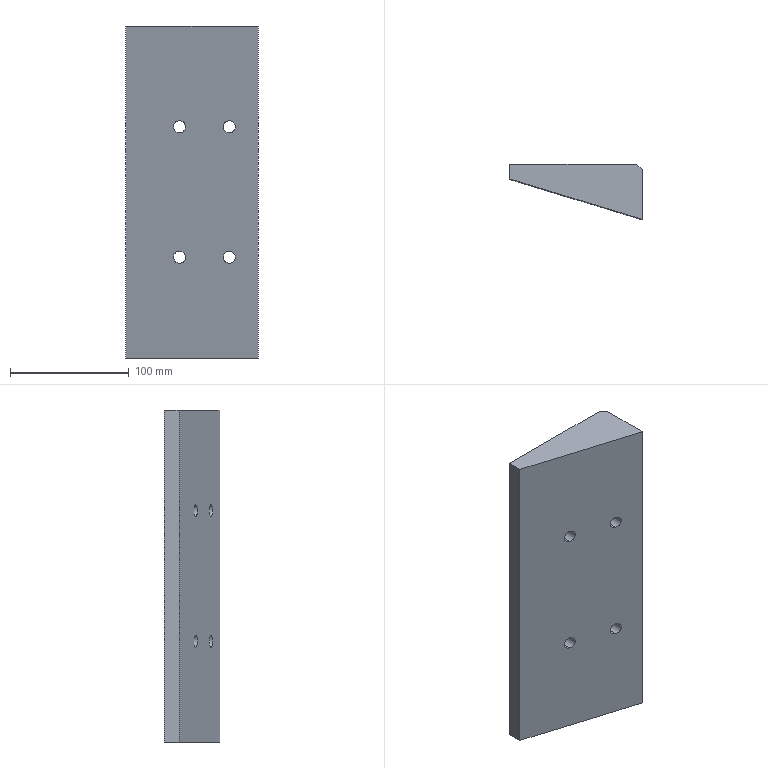Part | SolidWorks | features Extrusion 1, HoleWzd 1 | 1 solid | 15 faces | box 112 x 46.7 x 280 mm | volume 914034 mm3 | cylinder 8 | plane 7 | commonest cylinder face diameters 10.2 x8
STEP:
#1=CARTESIAN_POINT('',(45.5,-13.894,189.9));
#2=VERTEX_POINT('',#1);
#3=CARTESIAN_POINT('',(45.5,-13.894,200.1));
#4=VERTEX_POINT('',#3);
#5=CARTESIAN_POINT('',(45.5,-13.894,189.9));
#6=CARTESIAN_POINT('',(35.3,-10.779,189.9));
#7=CARTESIAN_POINT('',(35.3,-10.779,200.1));
#8=CARTESIAN_POINT('',(45.5,-13.894,200.1));
#9=(BOUNDED_CURVE()B_SPLINE_CURVE(3,(#5,#6,#7,#8),.UNSPECIFIED.,.F.,.T.)B_SPLINE_CURVE_WITH_KNOTS((4,4),(4.712,7.854),.UNSPECIFIED.)CURVE()GEOMETRIC_REPRESENTATION_ITEM()RATIONAL_B_SPLINE_CURVE((1.,0.3333,0.3333,1.))REPRESENTATION_ITEM(''));
#10=EDGE_CURVE('',#2,#4,#9,.T.);
#11=ORIENTED_EDGE('',*,*,#10,.F.);
#12=CARTESIAN_POINT('',(45.5,12.5,189.9));
#13=VERTEX_POINT('',#12);
#14=CARTESIAN_POINT('',(45.5,12.5,189.9));
#15=DIRECTION('',(0.,1.,0.));
#16=VECTOR('',#15,1000.);
#17=LINE('',#14,#16);
#18=EDGE_CURVE('',#2,#13,#17,.T.);
#19=ORIENTED_EDGE('',*,*,#18,.T.);
#20=CARTESIAN_POINT('',(45.5,12.5,200.1));
#21=VERTEX_POINT('',#20);
#22=CARTESIAN_POINT('',(45.5,12.5,195.));
#23=DIRECTION('',(0.,1.,0.));
#24=DIRECTION('',(0.,0.,1.));
#25=AXIS2_PLACEMENT_3D('',#22,#23,#24);
#26=CIRCLE('',#25,5.1);
#27=EDGE_CURVE('',#13,#21,#26,.T.);
#28=ORIENTED_EDGE('',*,*,#27,.T.);
#29=CARTESIAN_POINT('',(45.5,12.5,200.1));
#30=DIRECTION('',(0.,1.,0.));
#31=VECTOR('',#30,1000.);
#32=LINE('',#29,#31);
#33=EDGE_CURVE('',#4,#21,#32,.T.);
#34=ORIENTED_EDGE('',*,*,#33,.F.);
#35=EDGE_LOOP('',(#11,#19,#28,#34));
#36=FACE_OUTER_BOUND('',#35,.T.);
#37=CARTESIAN_POINT('',(45.5,12.5,195.));
#38=DIRECTION('',(0.,1.,0.));
#39=DIRECTION('',(0.,0.,1.));
#40=AXIS2_PLACEMENT_3D('',#37,#38,#39);
#41=CYLINDRICAL_SURFACE('',#40,5.1);
#42=ADVANCED_FACE('',(#36),#41,.F.);
#43=CARTESIAN_POINT('',(45.5,-13.894,79.9));
#44=VERTEX_POINT('',#43);
#45=CARTESIAN_POINT('',(45.5,-13.894,90.1));
#46=VERTEX_POINT('',#45);
#47=CARTESIAN_POINT('',(45.5,-13.894,79.9));
#48=CARTESIAN_POINT('',(35.3,-10.779,79.9));
#49=CARTESIAN_POINT('',(35.3,-10.779,90.1));
#50=CARTESIAN_POINT('',(45.5,-13.894,90.1));
#51=(BOUNDED_CURVE()B_SPLINE_CURVE(3,(#47,#48,#49,#50),.UNSPECIFIED.,.F.,.F.)B_SPLINE_CURVE_WITH_KNOTS((4,4),(4.712,7.854),.UNSPECIFIED.)CURVE()GEOMETRIC_REPRESENTATION_ITEM()RATIONAL_B_SPLINE_CURVE((1.,0.3333,0.3333,1.))REPRESENTATION_ITEM(''));
#52=EDGE_CURVE('',#44,#46,#51,.T.);
#53=ORIENTED_EDGE('',*,*,#52,.F.);
#54=CARTESIAN_POINT('',(45.5,12.5,79.9));
#55=VERTEX_POINT('',#54);
#56=CARTESIAN_POINT('',(45.5,12.5,79.9));
#57=DIRECTION('',(0.,1.,0.));
#58=VECTOR('',#57,1000.);
#59=LINE('',#56,#58);
#60=EDGE_CURVE('',#44,#55,#59,.T.);
#61=ORIENTED_EDGE('',*,*,#60,.T.);
#62=CARTESIAN_POINT('',(45.5,12.5,90.1));
#63=VERTEX_POINT('',#62);
#64=CARTESIAN_POINT('',(45.5,12.5,85.));
#65=DIRECTION('',(0.,1.,0.));
#66=DIRECTION('',(0.,0.,1.));
#67=AXIS2_PLACEMENT_3D('',#64,#65,#66);
#68=CIRCLE('',#67,5.1);
#69=EDGE_CURVE('',#55,#63,#68,.T.);
#70=ORIENTED_EDGE('',*,*,#69,.T.);
#71=CARTESIAN_POINT('',(45.5,12.5,90.1));
#72=DIRECTION('',(0.,1.,0.));
#73=VECTOR('',#72,1000.);
#74=LINE('',#71,#73);
#75=EDGE_CURVE('',#46,#63,#74,.T.);
#76=ORIENTED_EDGE('',*,*,#75,.F.);
#77=EDGE_LOOP('',(#53,#61,#70,#76));
#78=FACE_OUTER_BOUND('',#77,.T.);
#79=CARTESIAN_POINT('',(45.5,12.5,85.));
#80=DIRECTION('',(0.,1.,0.));
#81=DIRECTION('',(0.,0.,1.));
#82=AXIS2_PLACEMENT_3D('',#79,#80,#81);
#83=CYLINDRICAL_SURFACE('',#82,5.1);
#84=ADVANCED_FACE('',(#78),#83,.F.);
#85=CARTESIAN_POINT('',(87.5,-26.719,79.9));
#86=VERTEX_POINT('',#85);
#87=CARTESIAN_POINT('',(87.5,-26.719,90.1));
#88=VERTEX_POINT('',#87);
#89=CARTESIAN_POINT('',(87.5,-26.719,79.9));
#90=CARTESIAN_POINT('',(77.3,-23.604,79.9));
#91=CARTESIAN_POINT('',(77.3,-23.604,90.1));
#92=CARTESIAN_POINT('',(87.5,-26.719,90.1));
#93=(BOUNDED_CURVE()B_SPLINE_CURVE(3,(#89,#90,#91,#92),.UNSPECIFIED.,.F.,.F.)B_SPLINE_CURVE_WITH_KNOTS((4,4),(4.712,7.854),.UNSPECIFIED.)CURVE()GEOMETRIC_REPRESENTATION_ITEM()RATIONAL_B_SPLINE_CURVE((1.,0.3333,0.3333,1.))REPRESENTATION_ITEM(''));
#94=EDGE_CURVE('',#86,#88,#93,.T.);
#95=ORIENTED_EDGE('',*,*,#94,.F.);
#96=CARTESIAN_POINT('',(87.5,12.5,79.9));
#97=VERTEX_POINT('',#96);
#98=CARTESIAN_POINT('',(87.5,12.5,79.9));
#99=DIRECTION('',(0.,1.,0.));
#100=VECTOR('',#99,1000.);
#101=LINE('',#98,#100);
#102=EDGE_CURVE('',#86,#97,#101,.T.);
#103=ORIENTED_EDGE('',*,*,#102,.T.);
#104=CARTESIAN_POINT('',(87.5,12.5,90.1));
#105=VERTEX_POINT('',#104);
#106=CARTESIAN_POINT('',(87.5,12.5,85.));
#107=DIRECTION('',(0.,1.,0.));
#108=DIRECTION('',(0.,0.,1.));
#109=AXIS2_PLACEMENT_3D('',#106,#107,#108);
#110=CIRCLE('',#109,5.1);
#111=EDGE_CURVE('',#97,#105,#110,.T.);
#112=ORIENTED_EDGE('',*,*,#111,.T.);
#113=CARTESIAN_POINT('',(87.5,12.5,90.1));
#114=DIRECTION('',(0.,1.,0.));
#115=VECTOR('',#114,1000.);
#116=LINE('',#113,#115);
#117=EDGE_CURVE('',#88,#105,#116,.T.);
#118=ORIENTED_EDGE('',*,*,#117,.F.);
#119=EDGE_LOOP('',(#95,#103,#112,#118));
#120=FACE_OUTER_BOUND('',#119,.T.);
#121=CARTESIAN_POINT('',(87.5,12.5,85.));
#122=DIRECTION('',(0.,1.,0.));
#123=DIRECTION('',(0.,0.,1.));
#124=AXIS2_PLACEMENT_3D('',#121,#122,#123);
#125=CYLINDRICAL_SURFACE('',#124,5.1);
#126=ADVANCED_FACE('',(#120),#125,.F.);
#127=CARTESIAN_POINT('',(87.5,-26.719,189.9));
#128=VERTEX_POINT('',#127);
#129=CARTESIAN_POINT('',(87.5,-26.719,200.1));
#130=VERTEX_POINT('',#129);
#131=CARTESIAN_POINT('',(87.5,-26.719,189.9));
#132=CARTESIAN_POINT('',(77.3,-23.604,189.9));
#133=CARTESIAN_POINT('',(77.3,-23.604,200.1));
#134=CARTESIAN_POINT('',(87.5,-26.719,200.1));
#135=(BOUNDED_CURVE()B_SPLINE_CURVE(3,(#131,#132,#133,#134),.UNSPECIFIED.,.F.,.T.)B_SPLINE_CURVE_WITH_KNOTS((4,4),(4.712,7.854),.UNSPECIFIED.)CURVE()GEOMETRIC_REPRESENTATION_ITEM()RATIONAL_B_SPLINE_CURVE((1.,0.3333,0.3333,1.))REPRESENTATION_ITEM(''));
#136=EDGE_CURVE('',#128,#130,#135,.T.);
#137=ORIENTED_EDGE('',*,*,#136,.F.);
#138=CARTESIAN_POINT('',(87.5,12.5,189.9));
#139=VERTEX_POINT('',#138);
#140=CARTESIAN_POINT('',(87.5,12.5,189.9));
#141=DIRECTION('',(0.,1.,0.));
#142=VECTOR('',#141,1000.);
#143=LINE('',#140,#142);
#144=EDGE_CURVE('',#128,#139,#143,.T.);
#145=ORIENTED_EDGE('',*,*,#144,.T.);
#146=CARTESIAN_POINT('',(87.5,12.5,200.1));
#147=VERTEX_POINT('',#146);
#148=CARTESIAN_POINT('',(87.5,12.5,195.));
#149=DIRECTION('',(0.,1.,0.));
#150=DIRECTION('',(0.,0.,1.));
#151=AXIS2_PLACEMENT_3D('',#148,#149,#150);
#152=CIRCLE('',#151,5.1);
#153=EDGE_CURVE('',#139,#147,#152,.T.);
#154=ORIENTED_EDGE('',*,*,#153,.T.);
#155=CARTESIAN_POINT('',(87.5,12.5,200.1));
#156=DIRECTION('',(0.,1.,0.));
#157=VECTOR('',#156,1000.);
#158=LINE('',#155,#157);
#159=EDGE_CURVE('',#130,#147,#158,.T.);
#160=ORIENTED_EDGE('',*,*,#159,.F.);
#161=EDGE_LOOP('',(#137,#145,#154,#160));
#162=FACE_OUTER_BOUND('',#161,.T.);
#163=CARTESIAN_POINT('',(87.5,12.5,195.));
#164=DIRECTION('',(0.,1.,0.));
#165=DIRECTION('',(0.,0.,1.));
#166=AXIS2_PLACEMENT_3D('',#163,#164,#165);
#167=CYLINDRICAL_SURFACE('',#166,5.1);
#168=ADVANCED_FACE('',(#162),#167,.F.);
#169=CARTESIAN_POINT('',(45.5,-13.894,200.1));
#170=CARTESIAN_POINT('',(55.7,-17.008,200.1));
#171=CARTESIAN_POINT('',(55.7,-17.008,189.9));
#172=CARTESIAN_POINT('',(45.5,-13.894,189.9));
#173=(BOUNDED_CURVE()B_SPLINE_CURVE(3,(#169,#170,#171,#172),.UNSPECIFIED.,.F.,.T.)B_SPLINE_CURVE_WITH_KNOTS((4,4),(1.571,4.712),.UNSPECIFIED.)CURVE()GEOMETRIC_REPRESENTATION_ITEM()RATIONAL_B_SPLINE_CURVE((1.,0.3333,0.3333,1.))REPRESENTATION_ITEM(''));
#174=EDGE_CURVE('',#4,#2,#173,.T.);
#175=ORIENTED_EDGE('',*,*,#174,.T.);
#176=ORIENTED_EDGE('',*,*,#10,.T.);
#177=EDGE_LOOP('',(#175,#176));
#178=FACE_BOUND('',#177,.T.);
#179=CARTESIAN_POINT('',(45.5,-13.894,90.1));
#180=CARTESIAN_POINT('',(55.7,-17.008,90.1));
#181=CARTESIAN_POINT('',(55.7,-17.008,79.9));
#182=CARTESIAN_POINT('',(45.5,-13.894,79.9));
#183=(BOUNDED_CURVE()B_SPLINE_CURVE(3,(#179,#180,#181,#182),.UNSPECIFIED.,.F.,.F.)B_SPLINE_CURVE_WITH_KNOTS((4,4),(1.571,4.712),.UNSPECIFIED.)CURVE()GEOMETRIC_REPRESENTATION_ITEM()RATIONAL_B_SPLINE_CURVE((1.,0.3333,0.3333,1.))REPRESENTATION_ITEM(''));
#184=EDGE_CURVE('',#46,#44,#183,.T.);
#185=ORIENTED_EDGE('',*,*,#184,.T.);
#186=ORIENTED_EDGE('',*,*,#52,.T.);
#187=EDGE_LOOP('',(#185,#186));
#188=FACE_BOUND('',#187,.T.);
#189=CARTESIAN_POINT('',(87.5,-26.719,90.1));
#190=CARTESIAN_POINT('',(97.7,-29.833,90.1));
#191=CARTESIAN_POINT('',(97.7,-29.833,79.9));
#192=CARTESIAN_POINT('',(87.5,-26.719,79.9));
#193=(BOUNDED_CURVE()B_SPLINE_CURVE(3,(#189,#190,#191,#192),.UNSPECIFIED.,.F.,.T.)B_SPLINE_CURVE_WITH_KNOTS((4,4),(1.571,4.712),.UNSPECIFIED.)CURVE()GEOMETRIC_REPRESENTATION_ITEM()RATIONAL_B_SPLINE_CURVE((1.,0.3333,0.3333,1.))REPRESENTATION_ITEM(''));
#194=EDGE_CURVE('',#88,#86,#193,.T.);
#195=ORIENTED_EDGE('',*,*,#194,.T.);
#196=ORIENTED_EDGE('',*,*,#94,.T.);
#197=EDGE_LOOP('',(#195,#196));
#198=FACE_BOUND('',#197,.T.);
#199=CARTESIAN_POINT('',(87.5,-26.719,200.1));
#200=CARTESIAN_POINT('',(97.7,-29.833,200.1));
#201=CARTESIAN_POINT('',(97.7,-29.833,189.9));
#202=CARTESIAN_POINT('',(87.5,-26.719,189.9));
#203=(BOUNDED_CURVE()B_SPLINE_CURVE(3,(#199,#200,#201,#202),.UNSPECIFIED.,.F.,.T.)B_SPLINE_CURVE_WITH_KNOTS((4,4),(1.571,4.712),.UNSPECIFIED.)CURVE()GEOMETRIC_REPRESENTATION_ITEM()RATIONAL_B_SPLINE_CURVE((1.,0.3333,0.3333,1.))REPRESENTATION_ITEM(''));
#204=EDGE_CURVE('',#130,#128,#203,.T.);
#205=ORIENTED_EDGE('',*,*,#204,.T.);
#206=ORIENTED_EDGE('',*,*,#136,.T.);
#207=EDGE_LOOP('',(#205,#206));
#208=FACE_BOUND('',#207,.T.);
#209=CARTESIAN_POINT('',(0.,0.,0.));
#210=VERTEX_POINT('',#209);
#211=CARTESIAN_POINT('',(112.,-34.2,0.));
#212=VERTEX_POINT('',#211);
#213=CARTESIAN_POINT('',(112.,-34.2,0.));
#214=DIRECTION('',(0.9564,-0.292,0.));
#215=VECTOR('',#214,1000.);
#216=LINE('',#213,#215);
#217=EDGE_CURVE('',#210,#212,#216,.T.);
#218=ORIENTED_EDGE('',*,*,#217,.T.);
#219=CARTESIAN_POINT('',(112.,-34.2,280.));
#220=VERTEX_POINT('',#219);
#221=CARTESIAN_POINT('',(112.,-34.2,280.));
#222=DIRECTION('',(0.,0.,-1.));
#223=VECTOR('',#222,1000.);
#224=LINE('',#221,#223);
#225=EDGE_CURVE('',#220,#212,#224,.T.);
#226=ORIENTED_EDGE('',*,*,#225,.F.);
#227=CARTESIAN_POINT('',(0.,0.,280.));
#228=VERTEX_POINT('',#227);
#229=CARTESIAN_POINT('',(112.,-34.2,280.));
#230=DIRECTION('',(0.9564,-0.292,0.));
#231=VECTOR('',#230,1000.);
#232=LINE('',#229,#231);
#233=EDGE_CURVE('',#228,#220,#232,.T.);
#234=ORIENTED_EDGE('',*,*,#233,.F.);
#235=CARTESIAN_POINT('',(0.,0.,280.));
#236=DIRECTION('',(0.,0.,-1.));
#237=VECTOR('',#236,1000.);
#238=LINE('',#235,#237);
#239=EDGE_CURVE('',#228,#210,#238,.T.);
#240=ORIENTED_EDGE('',*,*,#239,.T.);
#241=EDGE_LOOP('',(#218,#226,#234,#240));
#242=FACE_OUTER_BOUND('',#241,.T.);
#243=CARTESIAN_POINT('',(112.,-34.2,280.));
#244=DIRECTION('',(0.292,0.9564,0.));
#245=DIRECTION('',(-0.9564,0.292,0.));
#246=AXIS2_PLACEMENT_3D('',#243,#244,#245);
#247=PLANE('',#246);
#248=ADVANCED_FACE('',(#178,#188,#198,#208,#242),#247,.F.);
#249=CARTESIAN_POINT('',(112.,7.5,0.));
#250=VERTEX_POINT('',#249);
#251=CARTESIAN_POINT('',(112.,7.5,0.));
#252=DIRECTION('',(0.,1.,0.));
#253=VECTOR('',#252,1000.);
#254=LINE('',#251,#253);
#255=EDGE_CURVE('',#212,#250,#254,.T.);
#256=ORIENTED_EDGE('',*,*,#255,.T.);
#257=CARTESIAN_POINT('',(112.,7.5,280.));
#258=VERTEX_POINT('',#257);
#259=CARTESIAN_POINT('',(112.,7.5,280.));
#260=DIRECTION('',(0.,0.,-1.));
#261=VECTOR('',#260,1000.);
#262=LINE('',#259,#261);
#263=EDGE_CURVE('',#258,#250,#262,.T.);
#264=ORIENTED_EDGE('',*,*,#263,.F.);
#265=CARTESIAN_POINT('',(112.,7.5,280.));
#266=DIRECTION('',(0.,1.,0.));
#267=VECTOR('',#266,1000.);
#268=LINE('',#265,#267);
#269=EDGE_CURVE('',#220,#258,#268,.T.);
#270=ORIENTED_EDGE('',*,*,#269,.F.);
#271=ORIENTED_EDGE('',*,*,#225,.T.);
#272=EDGE_LOOP('',(#256,#264,#270,#271));
#273=FACE_OUTER_BOUND('',#272,.T.);
#274=CARTESIAN_POINT('',(112.,7.5,280.));
#275=DIRECTION('',(-1.,0.,0.));
#276=DIRECTION('',(0.,0.,1.));
#277=AXIS2_PLACEMENT_3D('',#274,#275,#276);
#278=PLANE('',#277);
#279=ADVANCED_FACE('',(#273),#278,.F.);
#280=CARTESIAN_POINT('',(107.,12.5,0.));
#281=VERTEX_POINT('',#280);
#282=CARTESIAN_POINT('',(107.,12.5,0.));
#283=DIRECTION('',(-0.7071,0.7071,0.));
#284=VECTOR('',#283,1000.);
#285=LINE('',#282,#284);
#286=EDGE_CURVE('',#250,#281,#285,.T.);
#287=ORIENTED_EDGE('',*,*,#286,.T.);
#288=CARTESIAN_POINT('',(107.,12.5,280.));
#289=VERTEX_POINT('',#288);
#290=CARTESIAN_POINT('',(107.,12.5,280.));
#291=DIRECTION('',(0.,0.,-1.));
#292=VECTOR('',#291,1000.);
#293=LINE('',#290,#292);
#294=EDGE_CURVE('',#289,#281,#293,.T.);
#295=ORIENTED_EDGE('',*,*,#294,.F.);
#296=CARTESIAN_POINT('',(107.,12.5,280.));
#297=DIRECTION('',(-0.7071,0.7071,0.));
#298=VECTOR('',#297,1000.);
#299=LINE('',#296,#298);
#300=EDGE_CURVE('',#258,#289,#299,.T.);
#301=ORIENTED_EDGE('',*,*,#300,.F.);
#302=ORIENTED_EDGE('',*,*,#263,.T.);
#303=EDGE_LOOP('',(#287,#295,#301,#302));
#304=FACE_OUTER_BOUND('',#303,.T.);
#305=CARTESIAN_POINT('',(107.,12.5,280.));
#306=DIRECTION('',(-0.7071,-0.7071,0.));
#307=DIRECTION('',(0.7071,-0.7071,0.));
#308=AXIS2_PLACEMENT_3D('',#305,#306,#307);
#309=PLANE('',#308);
#310=ADVANCED_FACE('',(#304),#309,.F.);
#311=CARTESIAN_POINT('',(45.5,12.5,195.));
#312=DIRECTION('',(0.,1.,0.));
#313=DIRECTION('',(0.,0.,1.));
#314=AXIS2_PLACEMENT_3D('',#311,#312,#313);
#315=CIRCLE('',#314,5.1);
#316=EDGE_CURVE('',#21,#13,#315,.T.);
#317=ORIENTED_EDGE('',*,*,#316,.F.);
#318=ORIENTED_EDGE('',*,*,#27,.F.);
#319=EDGE_LOOP('',(#317,#318));
#320=FACE_BOUND('',#319,.T.);
#321=CARTESIAN_POINT('',(45.5,12.5,85.));
#322=DIRECTION('',(0.,1.,0.));
#323=DIRECTION('',(0.,0.,1.));
#324=AXIS2_PLACEMENT_3D('',#321,#322,#323);
#325=CIRCLE('',#324,5.1);
#326=EDGE_CURVE('',#63,#55,#325,.T.);
#327=ORIENTED_EDGE('',*,*,#326,.F.);
#328=ORIENTED_EDGE('',*,*,#69,.F.);
#329=EDGE_LOOP('',(#327,#328));
#330=FACE_BOUND('',#329,.T.);
#331=CARTESIAN_POINT('',(87.5,12.5,85.));
#332=DIRECTION('',(0.,1.,0.));
#333=DIRECTION('',(0.,0.,1.));
#334=AXIS2_PLACEMENT_3D('',#331,#332,#333);
#335=CIRCLE('',#334,5.1);
#336=EDGE_CURVE('',#105,#97,#335,.T.);
#337=ORIENTED_EDGE('',*,*,#336,.F.);
#338=ORIENTED_EDGE('',*,*,#111,.F.);
#339=EDGE_LOOP('',(#337,#338));
#340=FACE_BOUND('',#339,.T.);
#341=CARTESIAN_POINT('',(87.5,12.5,195.));
#342=DIRECTION('',(0.,1.,0.));
#343=DIRECTION('',(0.,0.,1.));
#344=AXIS2_PLACEMENT_3D('',#341,#342,#343);
#345=CIRCLE('',#344,5.1);
#346=EDGE_CURVE('',#147,#139,#345,.T.);
#347=ORIENTED_EDGE('',*,*,#346,.F.);
#348=ORIENTED_EDGE('',*,*,#153,.F.);
#349=EDGE_LOOP('',(#347,#348));
#350=FACE_BOUND('',#349,.T.);
#351=CARTESIAN_POINT('',(0.,12.5,0.));
#352=VERTEX_POINT('',#351);
#353=CARTESIAN_POINT('',(0.,12.5,0.));
#354=DIRECTION('',(-1.,0.,0.));
#355=VECTOR('',#354,1000.);
#356=LINE('',#353,#355);
#357=EDGE_CURVE('',#281,#352,#356,.T.);
#358=ORIENTED_EDGE('',*,*,#357,.T.);
#359=CARTESIAN_POINT('',(0.,12.5,280.));
#360=VERTEX_POINT('',#359);
#361=CARTESIAN_POINT('',(0.,12.5,280.));
#362=DIRECTION('',(0.,0.,-1.));
#363=VECTOR('',#362,1000.);
#364=LINE('',#361,#363);
#365=EDGE_CURVE('',#360,#352,#364,.T.);
#366=ORIENTED_EDGE('',*,*,#365,.F.);
#367=CARTESIAN_POINT('',(0.,12.5,280.));
#368=DIRECTION('',(-1.,0.,0.));
#369=VECTOR('',#368,1000.);
#370=LINE('',#367,#369);
#371=EDGE_CURVE('',#289,#360,#370,.T.);
#372=ORIENTED_EDGE('',*,*,#371,.F.);
#373=ORIENTED_EDGE('',*,*,#294,.T.);
#374=EDGE_LOOP('',(#358,#366,#372,#373));
#375=FACE_OUTER_BOUND('',#374,.T.);
#376=CARTESIAN_POINT('',(0.,12.5,280.));
#377=DIRECTION('',(0.,-1.,0.));
#378=DIRECTION('',(0.,0.,-1.));
#379=AXIS2_PLACEMENT_3D('',#376,#377,#378);
#380=PLANE('',#379);
#381=ADVANCED_FACE('',(#320,#330,#340,#350,#375),#380,.F.);
#382=CARTESIAN_POINT('',(0.,0.,0.));
#383=DIRECTION('',(0.,-1.,0.));
#384=VECTOR('',#383,1000.);
#385=LINE('',#382,#384);
#386=EDGE_CURVE('',#352,#210,#385,.T.);
#387=ORIENTED_EDGE('',*,*,#386,.T.);
#388=ORIENTED_EDGE('',*,*,#239,.F.);
#389=CARTESIAN_POINT('',(0.,0.,280.));
#390=DIRECTION('',(0.,-1.,0.));
#391=VECTOR('',#390,1000.);
#392=LINE('',#389,#391);
#393=EDGE_CURVE('',#360,#228,#392,.T.);
#394=ORIENTED_EDGE('',*,*,#393,.F.);
#395=ORIENTED_EDGE('',*,*,#365,.T.);
#396=EDGE_LOOP('',(#387,#388,#394,#395));
#397=FACE_OUTER_BOUND('',#396,.T.);
#398=CARTESIAN_POINT('',(0.,0.,280.));
#399=DIRECTION('',(1.,0.,0.));
#400=DIRECTION('',(0.,0.,-1.));
#401=AXIS2_PLACEMENT_3D('',#398,#399,#400);
#402=PLANE('',#401);
#403=ADVANCED_FACE('',(#397),#402,.F.);
#404=ORIENTED_EDGE('',*,*,#233,.T.);
#405=ORIENTED_EDGE('',*,*,#269,.T.);
#406=ORIENTED_EDGE('',*,*,#300,.T.);
#407=ORIENTED_EDGE('',*,*,#371,.T.);
#408=ORIENTED_EDGE('',*,*,#393,.T.);
#409=EDGE_LOOP('',(#404,#405,#406,#407,#408));
#410=FACE_OUTER_BOUND('',#409,.T.);
#411=CARTESIAN_POINT('',(0.,0.,280.));
#412=DIRECTION('',(0.,0.,-1.));
#413=DIRECTION('',(-1.,0.,0.));
#414=AXIS2_PLACEMENT_3D('',#411,#412,#413);
#415=PLANE('',#414);
#416=ADVANCED_FACE('',(#410),#415,.F.);
#417=ORIENTED_EDGE('',*,*,#217,.F.);
#418=ORIENTED_EDGE('',*,*,#386,.F.);
#419=ORIENTED_EDGE('',*,*,#357,.F.);
#420=ORIENTED_EDGE('',*,*,#286,.F.);
#421=ORIENTED_EDGE('',*,*,#255,.F.);
#422=EDGE_LOOP('',(#417,#418,#419,#420,#421));
#423=FACE_OUTER_BOUND('',#422,.T.);
#424=CARTESIAN_POINT('',(0.,0.,0.));
#425=DIRECTION('',(0.,0.,-1.));
#426=DIRECTION('',(-1.,0.,0.));
#427=AXIS2_PLACEMENT_3D('',#424,#425,#426);
#428=PLANE('',#427);
#429=ADVANCED_FACE('',(#423),#428,.T.);
#430=ORIENTED_EDGE('',*,*,#144,.F.);
#431=ORIENTED_EDGE('',*,*,#204,.F.);
#432=ORIENTED_EDGE('',*,*,#159,.T.);
#433=ORIENTED_EDGE('',*,*,#346,.T.);
#434=EDGE_LOOP('',(#430,#431,#432,#433));
#435=FACE_OUTER_BOUND('',#434,.T.);
#436=CARTESIAN_POINT('',(87.5,12.5,195.));
#437=DIRECTION('',(0.,1.,0.));
#438=DIRECTION('',(0.,0.,1.));
#439=AXIS2_PLACEMENT_3D('',#436,#437,#438);
#440=CYLINDRICAL_SURFACE('',#439,5.1);
#441=ADVANCED_FACE('',(#435),#440,.F.);
#442=ORIENTED_EDGE('',*,*,#102,.F.);
#443=ORIENTED_EDGE('',*,*,#194,.F.);
#444=ORIENTED_EDGE('',*,*,#117,.T.);
#445=ORIENTED_EDGE('',*,*,#336,.T.);
#446=EDGE_LOOP('',(#442,#443,#444,#445));
#447=FACE_OUTER_BOUND('',#446,.T.);
#448=CARTESIAN_POINT('',(87.5,12.5,85.));
#449=DIRECTION('',(0.,1.,0.));
#450=DIRECTION('',(0.,0.,1.));
#451=AXIS2_PLACEMENT_3D('',#448,#449,#450);
#452=CYLINDRICAL_SURFACE('',#451,5.1);
#453=ADVANCED_FACE('',(#447),#452,.F.);
#454=ORIENTED_EDGE('',*,*,#60,.F.);
#455=ORIENTED_EDGE('',*,*,#184,.F.);
#456=ORIENTED_EDGE('',*,*,#75,.T.);
#457=ORIENTED_EDGE('',*,*,#326,.T.);
#458=EDGE_LOOP('',(#454,#455,#456,#457));
#459=FACE_OUTER_BOUND('',#458,.T.);
#460=CARTESIAN_POINT('',(45.5,12.5,85.));
#461=DIRECTION('',(0.,1.,0.));
#462=DIRECTION('',(0.,0.,1.));
#463=AXIS2_PLACEMENT_3D('',#460,#461,#462);
#464=CYLINDRICAL_SURFACE('',#463,5.1);
#465=ADVANCED_FACE('',(#459),#464,.F.);
#466=ORIENTED_EDGE('',*,*,#18,.F.);
#467=ORIENTED_EDGE('',*,*,#174,.F.);
#468=ORIENTED_EDGE('',*,*,#33,.T.);
#469=ORIENTED_EDGE('',*,*,#316,.T.);
#470=EDGE_LOOP('',(#466,#467,#468,#469));
#471=FACE_OUTER_BOUND('',#470,.T.);
#472=CARTESIAN_POINT('',(45.5,12.5,195.));
#473=DIRECTION('',(0.,1.,0.));
#474=DIRECTION('',(0.,0.,1.));
#475=AXIS2_PLACEMENT_3D('',#472,#473,#474);
#476=CYLINDRICAL_SURFACE('',#475,5.1);
#477=ADVANCED_FACE('',(#471),#476,.F.);
#478=CLOSED_SHELL('',(#42,#84,#126,#168,#248,#279,#310,#381,#403,#416,#429,#441,#453,#465,#477));
#479=MANIFOLD_SOLID_BREP('',#478);
#480=CARTESIAN_POINT('',(0.,0.,0.));
#481=DIRECTION('',(0.,0.,1.));
#482=DIRECTION('',(1.,0.,0.));
#483=AXIS2_PLACEMENT_3D('',#480,#481,#482);
#484=(LENGTH_UNIT()NAMED_UNIT(*)SI_UNIT(.MILLI.,.METRE.));
#485=UNCERTAINTY_MEASURE_WITH_UNIT(LENGTH_MEASURE(0.00001),#484,'','');
#486=(NAMED_UNIT(*)PLANE_ANGLE_UNIT()SI_UNIT($,.RADIAN.));
#487=(NAMED_UNIT(*)SI_UNIT($,.STERADIAN.)SOLID_ANGLE_UNIT());
#488=(GEOMETRIC_REPRESENTATION_CONTEXT(3)GLOBAL_UNCERTAINTY_ASSIGNED_CONTEXT((#485))GLOBAL_UNIT_ASSIGNED_CONTEXT((#484,#486,#487))REPRESENTATION_CONTEXT('',''));
#489=ADVANCED_BREP_SHAPE_REPRESENTATION('',(#479,#483),#488);